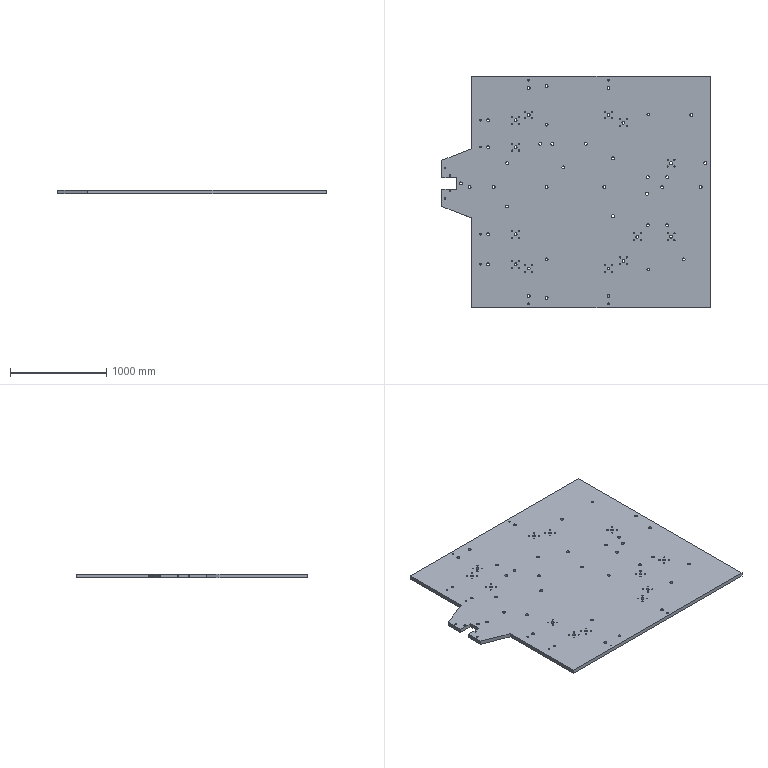Part | SolidWorks | features Extrusion 1 | 2 solids | 248 faces | box 2789 x 2400 x 40 mm | volume 242886322 mm3 | cylinder 232 | plane 16 | commonest cylinder face diameters 12 x104 30 x102 16 x24 10 x2